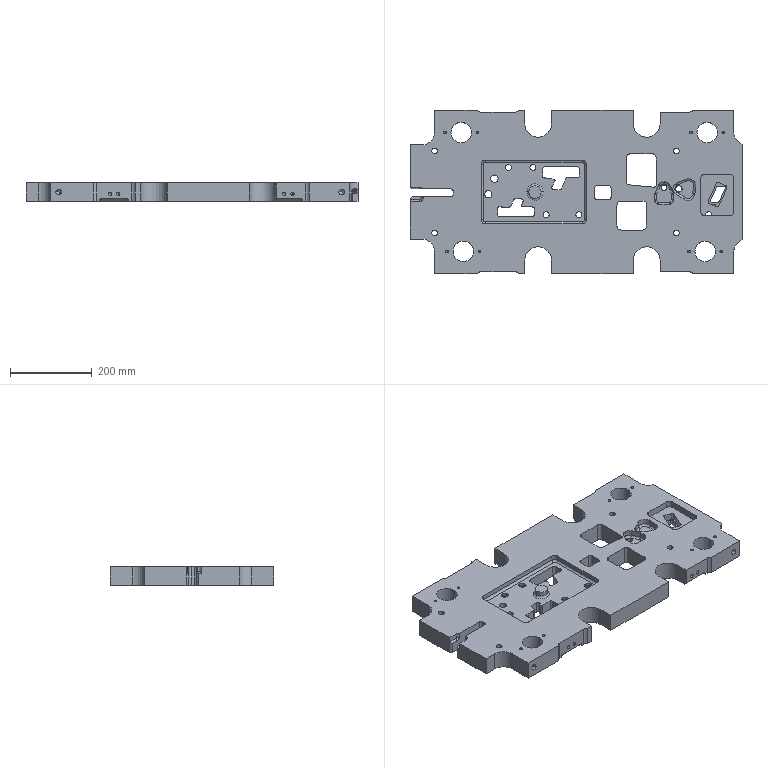Part | CATIA | 1 solid | 632 faces | box 810 x 400 x 45 mm | volume 9884776 mm3 | cylinder 313 | plane 168 | cone 76 | torus 52 | other 14 | sphere 7 | spline 2 | commonest cylinder face diameters 10 x78 18 x36 6 x35 11 x28 20 x22 14 x18